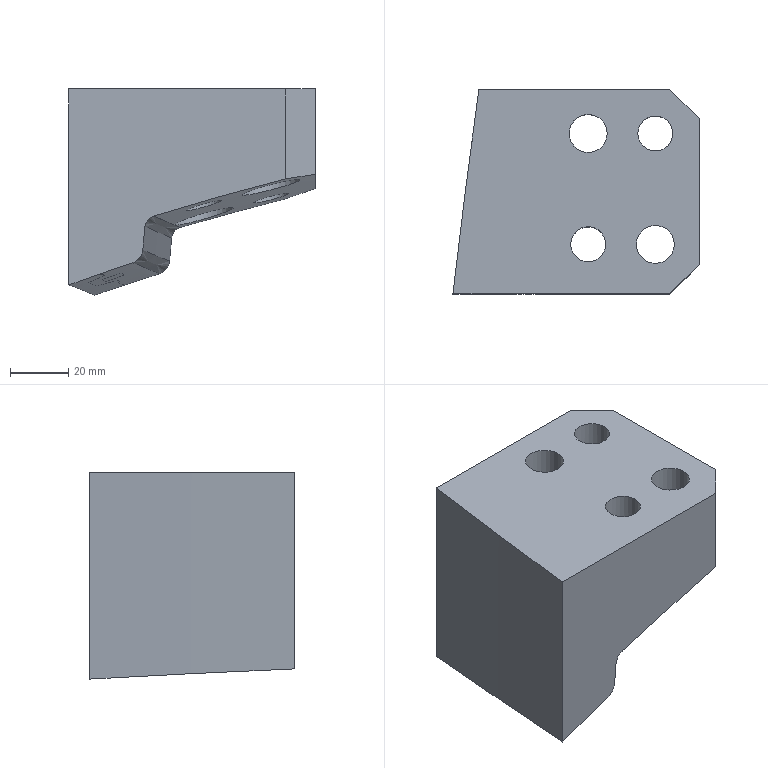Part | NX | features MAIN_BODY 2 | 1 solid | 23 faces | box 84.347 x 70 x 70.632 mm | volume 234093 mm3 | spline 9 | plane 8 | cylinder 6 | commonest cylinder face diameters 12 x2 13 x2 20 x2